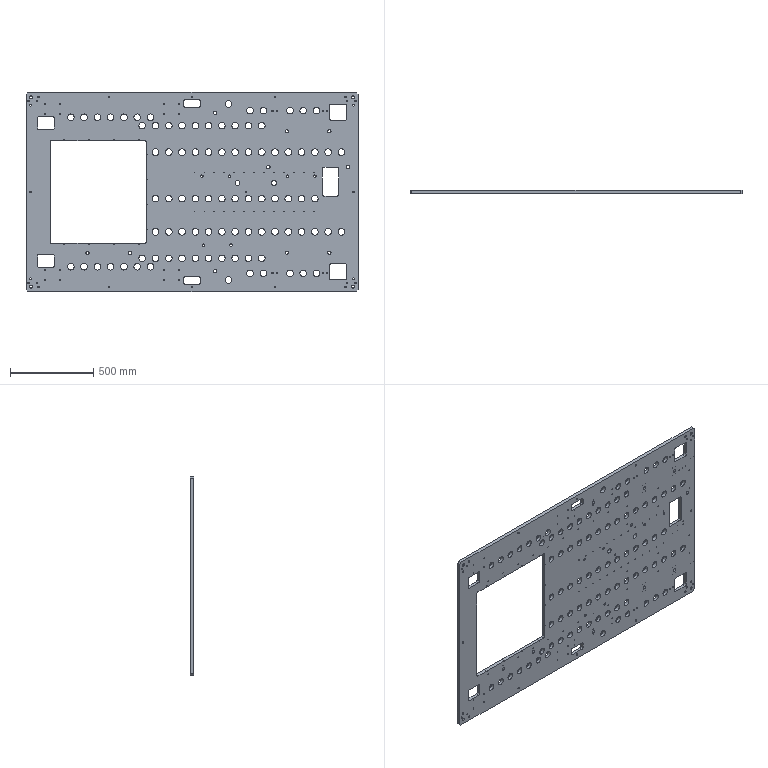Part | NX | 1 solid | 544 faces | box 2000 x 20 x 1200 mm | volume 37068890 mm3 | cylinder 366 | cone 111 | plane 67 | commonest cylinder face diameters 40 x89 5 x73 4.2 x42 20 x42 3.3 x30 11 x25